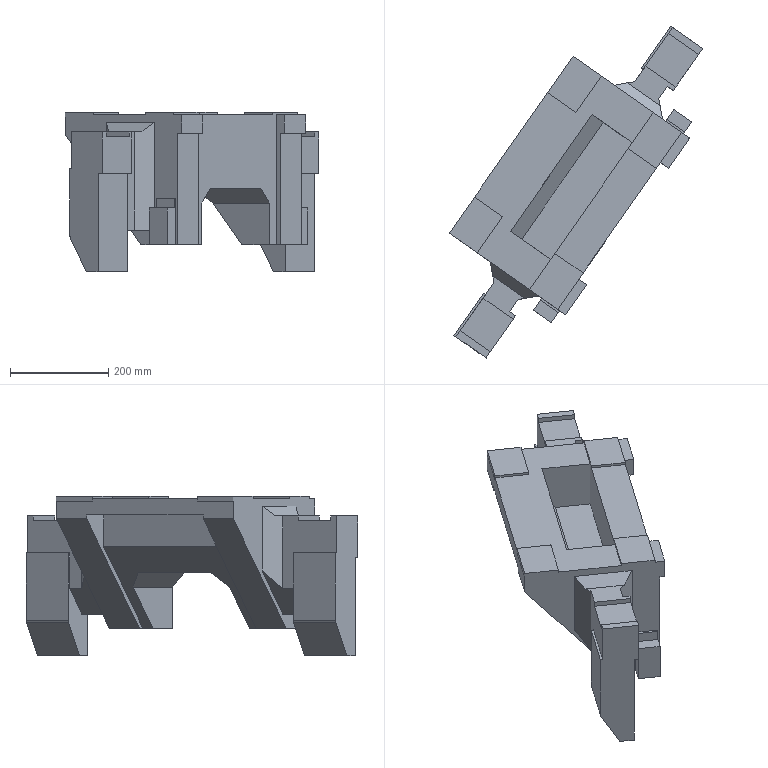Part | NX | features solid 2 | 1 solid | 110 faces | box 516.895 x 676.633 x 325 mm | volume 20803515 mm3 | plane 103 | cylinder 4 | spline 3 | commonest cylinder face diameters 20 x2 65 x2